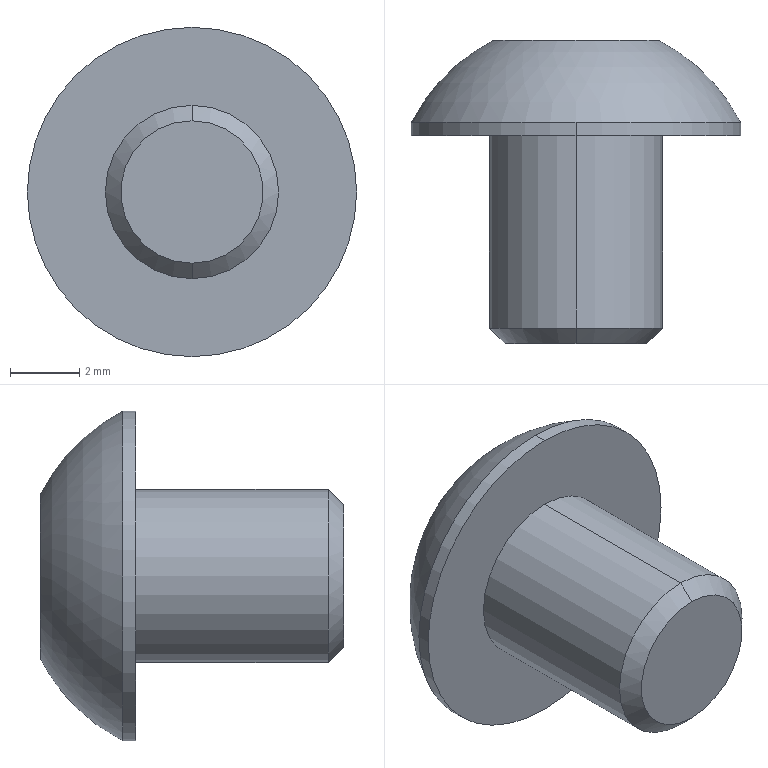Part | SolidWorks | features BaseBody 1 | 1 solid | 17 faces | box 9.5 x 8.75 x 9.5 mm | volume 242.513 mm3 | plane 10 | cylinder 4 | cone 2 | sphere 1 | commonest cylinder face diameters 5 x2 9.5 x2
STEP:
#1=CARTESIAN_POINT('',(0.,-6.,-2.055));
#2=VERTEX_POINT('',#1);
#3=CARTESIAN_POINT('',(0.,-6.,2.055));
#4=VERTEX_POINT('',#3);
#5=CARTESIAN_POINT('',(0.,-6.,0.));
#6=DIRECTION('',(0.,-1.,0.));
#7=DIRECTION('',(0.,0.,-1.));
#8=AXIS2_PLACEMENT_3D('',#5,#6,#7);
#9=CIRCLE('',#8,2.055);
#10=EDGE_CURVE('',#2,#4,#9,.T.);
#11=ORIENTED_EDGE('',*,*,#10,.F.);
#12=CARTESIAN_POINT('',(0.,-5.555,-2.5));
#13=VERTEX_POINT('',#12);
#14=CARTESIAN_POINT('',(0.,-6.,-2.055));
#15=DIRECTION('',(0.,0.7071,-0.7071));
#16=VECTOR('',#15,1000.);
#17=LINE('',#14,#16);
#18=EDGE_CURVE('',#2,#13,#17,.T.);
#19=ORIENTED_EDGE('',*,*,#18,.T.);
#20=CARTESIAN_POINT('',(0.,-5.555,2.5));
#21=VERTEX_POINT('',#20);
#22=CARTESIAN_POINT('',(0.,-5.555,0.));
#23=DIRECTION('',(0.,1.,0.));
#24=DIRECTION('',(0.,0.,-1.));
#25=AXIS2_PLACEMENT_3D('',#22,#23,#24);
#26=CIRCLE('',#25,2.5);
#27=EDGE_CURVE('',#21,#13,#26,.T.);
#28=ORIENTED_EDGE('',*,*,#27,.F.);
#29=CARTESIAN_POINT('',(0.,-6.,2.055));
#30=DIRECTION('',(0.,0.7071,0.7071));
#31=VECTOR('',#30,1000.);
#32=LINE('',#29,#31);
#33=EDGE_CURVE('',#4,#21,#32,.T.);
#34=ORIENTED_EDGE('',*,*,#33,.F.);
#35=EDGE_LOOP('',(#11,#19,#28,#34));
#36=FACE_OUTER_BOUND('',#35,.T.);
#37=CARTESIAN_POINT('',(0.,-6.,0.));
#38=DIRECTION('',(0.,1.,0.));
#39=DIRECTION('',(0.,0.,1.));
#40=AXIS2_PLACEMENT_3D('',#37,#38,#39);
#41=CONICAL_SURFACE('',#40,2.055,0.7854);
#42=ADVANCED_FACE('',(#36),#41,.T.);
#43=ORIENTED_EDGE('',*,*,#27,.T.);
#44=CARTESIAN_POINT('',(0.,0.,-2.5));
#45=VERTEX_POINT('',#44);
#46=CARTESIAN_POINT('',(0.,-6.,-2.5));
#47=DIRECTION('',(0.,1.,0.));
#48=VECTOR('',#47,1000.);
#49=LINE('',#46,#48);
#50=EDGE_CURVE('',#13,#45,#49,.T.);
#51=ORIENTED_EDGE('',*,*,#50,.T.);
#52=CARTESIAN_POINT('',(0.,0.,2.5));
#53=VERTEX_POINT('',#52);
#54=CARTESIAN_POINT('',(0.,0.,0.));
#55=DIRECTION('',(0.,-1.,0.));
#56=DIRECTION('',(0.,0.,1.));
#57=AXIS2_PLACEMENT_3D('',#54,#55,#56);
#58=CIRCLE('',#57,2.5);
#59=EDGE_CURVE('',#45,#53,#58,.T.);
#60=ORIENTED_EDGE('',*,*,#59,.T.);
#61=CARTESIAN_POINT('',(0.,-6.,2.5));
#62=DIRECTION('',(0.,1.,0.));
#63=VECTOR('',#62,1000.);
#64=LINE('',#61,#63);
#65=EDGE_CURVE('',#21,#53,#64,.T.);
#66=ORIENTED_EDGE('',*,*,#65,.F.);
#67=EDGE_LOOP('',(#43,#51,#60,#66));
#68=FACE_OUTER_BOUND('',#67,.T.);
#69=CARTESIAN_POINT('',(0.,-6.,0.));
#70=DIRECTION('',(0.,1.,0.));
#71=DIRECTION('',(0.,0.,1.));
#72=AXIS2_PLACEMENT_3D('',#69,#70,#71);
#73=CYLINDRICAL_SURFACE('',#72,2.5);
#74=ADVANCED_FACE('',(#68),#73,.T.);
#75=CARTESIAN_POINT('',(0.,0.38,-4.75));
#76=VERTEX_POINT('',#75);
#77=CARTESIAN_POINT('',(0.,0.38,4.75));
#78=VERTEX_POINT('',#77);
#79=CARTESIAN_POINT('',(0.,0.38,0.));
#80=DIRECTION('',(0.,-1.,0.));
#81=DIRECTION('',(0.,0.,-1.));
#82=AXIS2_PLACEMENT_3D('',#79,#80,#81);
#83=CIRCLE('',#82,4.75);
#84=EDGE_CURVE('',#76,#78,#83,.T.);
#85=ORIENTED_EDGE('',*,*,#84,.T.);
#86=CARTESIAN_POINT('',(0.,0.,4.75));
#87=VERTEX_POINT('',#86);
#88=CARTESIAN_POINT('',(0.,2.75,4.75));
#89=DIRECTION('',(0.,-1.,0.));
#90=VECTOR('',#89,1000.);
#91=LINE('',#88,#90);
#92=EDGE_CURVE('',#78,#87,#91,.T.);
#93=ORIENTED_EDGE('',*,*,#92,.T.);
#94=CARTESIAN_POINT('',(0.,0.,-4.75));
#95=VERTEX_POINT('',#94);
#96=CARTESIAN_POINT('',(0.,0.,0.));
#97=DIRECTION('',(0.,1.,0.));
#98=DIRECTION('',(0.,0.,1.));
#99=AXIS2_PLACEMENT_3D('',#96,#97,#98);
#100=CIRCLE('',#99,4.75);
#101=EDGE_CURVE('',#87,#95,#100,.T.);
#102=ORIENTED_EDGE('',*,*,#101,.T.);
#103=CARTESIAN_POINT('',(0.,2.75,-4.75));
#104=DIRECTION('',(0.,-1.,0.));
#105=VECTOR('',#104,1000.);
#106=LINE('',#103,#105);
#107=EDGE_CURVE('',#76,#95,#106,.T.);
#108=ORIENTED_EDGE('',*,*,#107,.F.);
#109=EDGE_LOOP('',(#85,#93,#102,#108));
#110=FACE_OUTER_BOUND('',#109,.T.);
#111=CARTESIAN_POINT('',(0.,2.75,0.));
#112=DIRECTION('',(0.,-1.,0.));
#113=DIRECTION('',(0.,0.,-1.));
#114=AXIS2_PLACEMENT_3D('',#111,#112,#113);
#115=CYLINDRICAL_SURFACE('',#114,4.75);
#116=ADVANCED_FACE('',(#110),#115,.T.);
#117=CARTESIAN_POINT('',(0.8862,2.75,1.535));
#118=VERTEX_POINT('',#117);
#119=CARTESIAN_POINT('',(1.772,2.75,0.));
#120=VERTEX_POINT('',#119);
#121=CARTESIAN_POINT('',(0.8862,2.75,1.535));
#122=DIRECTION('',(0.5,0.,-0.866));
#123=VECTOR('',#122,1000.);
#124=LINE('',#121,#123);
#125=EDGE_CURVE('',#118,#120,#124,.T.);
#126=ORIENTED_EDGE('',*,*,#125,.F.);
#127=CARTESIAN_POINT('',(-0.8862,2.75,1.535));
#128=VERTEX_POINT('',#127);
#129=CARTESIAN_POINT('',(-0.8862,2.75,1.535));
#130=DIRECTION('',(1.,0.,0.));
#131=VECTOR('',#130,1000.);
#132=LINE('',#129,#131);
#133=EDGE_CURVE('',#128,#118,#132,.T.);
#134=ORIENTED_EDGE('',*,*,#133,.F.);
#135=CARTESIAN_POINT('',(-1.772,2.75,0.));
#136=VERTEX_POINT('',#135);
#137=CARTESIAN_POINT('',(-1.772,2.75,0.));
#138=DIRECTION('',(0.5,0.,0.866));
#139=VECTOR('',#138,1000.);
#140=LINE('',#137,#139);
#141=EDGE_CURVE('',#136,#128,#140,.T.);
#142=ORIENTED_EDGE('',*,*,#141,.F.);
#143=CARTESIAN_POINT('',(-0.8862,2.75,-1.535));
#144=VERTEX_POINT('',#143);
#145=CARTESIAN_POINT('',(-0.8862,2.75,-1.535));
#146=DIRECTION('',(-0.5,0.,0.866));
#147=VECTOR('',#146,1000.);
#148=LINE('',#145,#147);
#149=EDGE_CURVE('',#144,#136,#148,.T.);
#150=ORIENTED_EDGE('',*,*,#149,.F.);
#151=CARTESIAN_POINT('',(0.8862,2.75,-1.535));
#152=VERTEX_POINT('',#151);
#153=CARTESIAN_POINT('',(0.8862,2.75,-1.535));
#154=DIRECTION('',(-1.,0.,0.));
#155=VECTOR('',#154,1000.);
#156=LINE('',#153,#155);
#157=EDGE_CURVE('',#152,#144,#156,.T.);
#158=ORIENTED_EDGE('',*,*,#157,.F.);
#159=CARTESIAN_POINT('',(1.772,2.75,0.));
#160=DIRECTION('',(-0.5,0.,-0.866));
#161=VECTOR('',#160,1000.);
#162=LINE('',#159,#161);
#163=EDGE_CURVE('',#120,#152,#162,.T.);
#164=ORIENTED_EDGE('',*,*,#163,.F.);
#165=EDGE_LOOP('',(#126,#134,#142,#150,#158,#164));
#166=FACE_BOUND('',#165,.T.);
#167=CARTESIAN_POINT('',(0.,2.75,-2.375));
#168=VERTEX_POINT('',#167);
#169=CARTESIAN_POINT('',(0.,2.75,2.375));
#170=VERTEX_POINT('',#169);
#171=CARTESIAN_POINT('',(0.,2.75,0.));
#172=DIRECTION('',(0.,-1.,0.));
#173=DIRECTION('',(0.,0.,-1.));
#174=AXIS2_PLACEMENT_3D('',#171,#172,#173);
#175=CIRCLE('',#174,2.375);
#176=EDGE_CURVE('',#168,#170,#175,.T.);
#177=ORIENTED_EDGE('',*,*,#176,.F.);
#178=CARTESIAN_POINT('',(0.,2.75,0.));
#179=DIRECTION('',(0.,-1.,0.));
#180=DIRECTION('',(0.,0.,-1.));
#181=AXIS2_PLACEMENT_3D('',#178,#179,#180);
#182=CIRCLE('',#181,2.375);
#183=EDGE_CURVE('',#170,#168,#182,.T.);
#184=ORIENTED_EDGE('',*,*,#183,.F.);
#185=EDGE_LOOP('',(#177,#184));
#186=FACE_OUTER_BOUND('',#185,.T.);
#187=CARTESIAN_POINT('',(0.,2.75,0.));
#188=DIRECTION('',(0.,1.,0.));
#189=DIRECTION('',(1.,0.,0.));
#190=AXIS2_PLACEMENT_3D('',#187,#188,#189);
#191=PLANE('',#190);
#192=ADVANCED_FACE('',(#166,#186),#191,.T.);
#193=ORIENTED_EDGE('',*,*,#125,.T.);
#194=CARTESIAN_POINT('',(1.772,1.19,0.));
#195=VERTEX_POINT('',#194);
#196=CARTESIAN_POINT('',(1.772,1.19,0.));
#197=DIRECTION('',(0.,1.,0.));
#198=VECTOR('',#197,1000.);
#199=LINE('',#196,#198);
#200=EDGE_CURVE('',#195,#120,#199,.T.);
#201=ORIENTED_EDGE('',*,*,#200,.F.);
#202=CARTESIAN_POINT('',(0.8862,1.19,1.535));
#203=VERTEX_POINT('',#202);
#204=CARTESIAN_POINT('',(0.8862,1.19,1.535));
#205=DIRECTION('',(0.5,0.,-0.866));
#206=VECTOR('',#205,1000.);
#207=LINE('',#204,#206);
#208=EDGE_CURVE('',#203,#195,#207,.T.);
#209=ORIENTED_EDGE('',*,*,#208,.F.);
#210=CARTESIAN_POINT('',(0.8862,1.19,1.535));
#211=DIRECTION('',(0.,1.,0.));
#212=VECTOR('',#211,1000.);
#213=LINE('',#210,#212);
#214=EDGE_CURVE('',#203,#118,#213,.T.);
#215=ORIENTED_EDGE('',*,*,#214,.T.);
#216=EDGE_LOOP('',(#193,#201,#209,#215));
#217=FACE_OUTER_BOUND('',#216,.T.);
#218=CARTESIAN_POINT('',(0.8862,1.19,1.535));
#219=DIRECTION('',(0.866,0.,0.5));
#220=DIRECTION('',(0.,-1.,0.));
#221=AXIS2_PLACEMENT_3D('',#218,#219,#220);
#222=PLANE('',#221);
#223=ADVANCED_FACE('',(#217),#222,.F.);
#224=ORIENTED_EDGE('',*,*,#133,.T.);
#225=ORIENTED_EDGE('',*,*,#214,.F.);
#226=CARTESIAN_POINT('',(-0.8862,1.19,1.535));
#227=VERTEX_POINT('',#226);
#228=CARTESIAN_POINT('',(-0.8862,1.19,1.535));
#229=DIRECTION('',(1.,0.,0.));
#230=VECTOR('',#229,1000.);
#231=LINE('',#228,#230);
#232=EDGE_CURVE('',#227,#203,#231,.T.);
#233=ORIENTED_EDGE('',*,*,#232,.F.);
#234=CARTESIAN_POINT('',(-0.8862,1.19,1.535));
#235=DIRECTION('',(0.,1.,0.));
#236=VECTOR('',#235,1000.);
#237=LINE('',#234,#236);
#238=EDGE_CURVE('',#227,#128,#237,.T.);
#239=ORIENTED_EDGE('',*,*,#238,.T.);
#240=EDGE_LOOP('',(#224,#225,#233,#239));
#241=FACE_OUTER_BOUND('',#240,.T.);
#242=CARTESIAN_POINT('',(-0.8862,1.19,1.535));
#243=DIRECTION('',(0.,0.,1.));
#244=DIRECTION('',(1.,0.,0.));
#245=AXIS2_PLACEMENT_3D('',#242,#243,#244);
#246=PLANE('',#245);
#247=ADVANCED_FACE('',(#241),#246,.F.);
#248=ORIENTED_EDGE('',*,*,#141,.T.);
#249=ORIENTED_EDGE('',*,*,#238,.F.);
#250=CARTESIAN_POINT('',(-1.772,1.19,0.));
#251=VERTEX_POINT('',#250);
#252=CARTESIAN_POINT('',(-1.772,1.19,0.));
#253=DIRECTION('',(0.5,0.,0.866));
#254=VECTOR('',#253,1000.);
#255=LINE('',#252,#254);
#256=EDGE_CURVE('',#251,#227,#255,.T.);
#257=ORIENTED_EDGE('',*,*,#256,.F.);
#258=CARTESIAN_POINT('',(-1.772,1.19,0.));
#259=DIRECTION('',(0.,1.,0.));
#260=VECTOR('',#259,1000.);
#261=LINE('',#258,#260);
#262=EDGE_CURVE('',#251,#136,#261,.T.);
#263=ORIENTED_EDGE('',*,*,#262,.T.);
#264=EDGE_LOOP('',(#248,#249,#257,#263));
#265=FACE_OUTER_BOUND('',#264,.T.);
#266=CARTESIAN_POINT('',(-1.772,1.19,0.));
#267=DIRECTION('',(-0.866,0.,0.5));
#268=DIRECTION('',(0.,1.,0.));
#269=AXIS2_PLACEMENT_3D('',#266,#267,#268);
#270=PLANE('',#269);
#271=ADVANCED_FACE('',(#265),#270,.F.);
#272=ORIENTED_EDGE('',*,*,#149,.T.);
#273=ORIENTED_EDGE('',*,*,#262,.F.);
#274=CARTESIAN_POINT('',(-0.8862,1.19,-1.535));
#275=VERTEX_POINT('',#274);
#276=CARTESIAN_POINT('',(-0.8862,1.19,-1.535));
#277=DIRECTION('',(-0.5,0.,0.866));
#278=VECTOR('',#277,1000.);
#279=LINE('',#276,#278);
#280=EDGE_CURVE('',#275,#251,#279,.T.);
#281=ORIENTED_EDGE('',*,*,#280,.F.);
#282=CARTESIAN_POINT('',(-0.8862,1.19,-1.535));
#283=DIRECTION('',(0.,1.,0.));
#284=VECTOR('',#283,1000.);
#285=LINE('',#282,#284);
#286=EDGE_CURVE('',#275,#144,#285,.T.);
#287=ORIENTED_EDGE('',*,*,#286,.T.);
#288=EDGE_LOOP('',(#272,#273,#281,#287));
#289=FACE_OUTER_BOUND('',#288,.T.);
#290=CARTESIAN_POINT('',(-0.8862,1.19,-1.535));
#291=DIRECTION('',(-0.866,0.,-0.5));
#292=DIRECTION('',(-0.5,0.,0.866));
#293=AXIS2_PLACEMENT_3D('',#290,#291,#292);
#294=PLANE('',#293);
#295=ADVANCED_FACE('',(#289),#294,.F.);
#296=ORIENTED_EDGE('',*,*,#157,.T.);
#297=ORIENTED_EDGE('',*,*,#286,.F.);
#298=CARTESIAN_POINT('',(0.8862,1.19,-1.535));
#299=VERTEX_POINT('',#298);
#300=CARTESIAN_POINT('',(0.8862,1.19,-1.535));
#301=DIRECTION('',(-1.,0.,0.));
#302=VECTOR('',#301,1000.);
#303=LINE('',#300,#302);
#304=EDGE_CURVE('',#299,#275,#303,.T.);
#305=ORIENTED_EDGE('',*,*,#304,.F.);
#306=CARTESIAN_POINT('',(0.8862,1.19,-1.535));
#307=DIRECTION('',(0.,1.,0.));
#308=VECTOR('',#307,1000.);
#309=LINE('',#306,#308);
#310=EDGE_CURVE('',#299,#152,#309,.T.);
#311=ORIENTED_EDGE('',*,*,#310,.T.);
#312=EDGE_LOOP('',(#296,#297,#305,#311));
#313=FACE_OUTER_BOUND('',#312,.T.);
#314=CARTESIAN_POINT('',(0.8862,1.19,-1.535));
#315=DIRECTION('',(0.,0.,-1.));
#316=DIRECTION('',(-1.,0.,0.));
#317=AXIS2_PLACEMENT_3D('',#314,#315,#316);
#318=PLANE('',#317);
#319=ADVANCED_FACE('',(#313),#318,.F.);
#320=ORIENTED_EDGE('',*,*,#163,.T.);
#321=ORIENTED_EDGE('',*,*,#310,.F.);
#322=CARTESIAN_POINT('',(1.772,1.19,0.));
#323=DIRECTION('',(-0.5,0.,-0.866));
#324=VECTOR('',#323,1000.);
#325=LINE('',#322,#324);
#326=EDGE_CURVE('',#195,#299,#325,.T.);
#327=ORIENTED_EDGE('',*,*,#326,.F.);
#328=ORIENTED_EDGE('',*,*,#200,.T.);
#329=EDGE_LOOP('',(#320,#321,#327,#328));
#330=FACE_OUTER_BOUND('',#329,.T.);
#331=CARTESIAN_POINT('',(1.772,1.19,0.));
#332=DIRECTION('',(0.866,0.,-0.5));
#333=DIRECTION('',(0.,-1.,0.));
#334=AXIS2_PLACEMENT_3D('',#331,#332,#333);
#335=PLANE('',#334);
#336=ADVANCED_FACE('',(#330),#335,.F.);
#337=ORIENTED_EDGE('',*,*,#208,.T.);
#338=ORIENTED_EDGE('',*,*,#326,.T.);
#339=ORIENTED_EDGE('',*,*,#304,.T.);
#340=ORIENTED_EDGE('',*,*,#280,.T.);
#341=ORIENTED_EDGE('',*,*,#256,.T.);
#342=ORIENTED_EDGE('',*,*,#232,.T.);
#343=EDGE_LOOP('',(#337,#338,#339,#340,#341,#342));
#344=FACE_OUTER_BOUND('',#343,.T.);
#345=CARTESIAN_POINT('',(0.,1.19,0.));
#346=DIRECTION('',(0.,1.,0.));
#347=DIRECTION('',(1.,0.,0.));
#348=AXIS2_PLACEMENT_3D('',#345,#346,#347);
#349=PLANE('',#348);
#350=ADVANCED_FACE('',(#344),#349,.T.);
#351=CARTESIAN_POINT('',(0.,-6.,0.));
#352=DIRECTION('',(0.,-1.,0.));
#353=DIRECTION('',(0.,0.,-1.));
#354=AXIS2_PLACEMENT_3D('',#351,#352,#353);
#355=CIRCLE('',#354,2.055);
#356=EDGE_CURVE('',#4,#2,#355,.T.);
#357=ORIENTED_EDGE('',*,*,#356,.T.);
#358=ORIENTED_EDGE('',*,*,#10,.T.);
#359=EDGE_LOOP('',(#357,#358));
#360=FACE_OUTER_BOUND('',#359,.T.);
#361=CARTESIAN_POINT('',(0.,-6.,0.));
#362=DIRECTION('',(0.,-1.,0.));
#363=DIRECTION('',(0.,0.,-1.));
#364=AXIS2_PLACEMENT_3D('',#361,#362,#363);
#365=PLANE('',#364);
#366=ADVANCED_FACE('',(#360),#365,.T.);
#367=CARTESIAN_POINT('',(0.,0.,0.));
#368=DIRECTION('',(0.,-1.,0.));
#369=DIRECTION('',(0.,0.,1.));
#370=AXIS2_PLACEMENT_3D('',#367,#368,#369);
#371=CIRCLE('',#370,2.5);
#372=EDGE_CURVE('',#53,#45,#371,.T.);
#373=ORIENTED_EDGE('',*,*,#372,.F.);
#374=ORIENTED_EDGE('',*,*,#59,.F.);
#375=EDGE_LOOP('',(#373,#374));
#376=FACE_BOUND('',#375,.T.);
#377=CARTESIAN_POINT('',(0.,0.,0.));
#378=DIRECTION('',(0.,1.,0.));
#379=DIRECTION('',(0.,0.,1.));
#380=AXIS2_PLACEMENT_3D('',#377,#378,#379);
#381=CIRCLE('',#380,4.75);
#382=EDGE_CURVE('',#95,#87,#381,.T.);
#383=ORIENTED_EDGE('',*,*,#382,.F.);
#384=ORIENTED_EDGE('',*,*,#101,.F.);
#385=EDGE_LOOP('',(#383,#384));
#386=FACE_OUTER_BOUND('',#385,.T.);
#387=CARTESIAN_POINT('',(0.,0.,0.));
#388=DIRECTION('',(0.,1.,0.));
#389=DIRECTION('',(1.,0.,0.));
#390=AXIS2_PLACEMENT_3D('',#387,#388,#389);
#391=PLANE('',#390);
#392=ADVANCED_FACE('',(#376,#386),#391,.F.);
#393=ORIENTED_EDGE('',*,*,#92,.F.);
#394=CARTESIAN_POINT('',(0.,0.38,0.));
#395=DIRECTION('',(0.,-1.,0.));
#396=DIRECTION('',(0.,0.,-1.));
#397=AXIS2_PLACEMENT_3D('',#394,#395,#396);
#398=CIRCLE('',#397,4.75);
#399=EDGE_CURVE('',#78,#76,#398,.T.);
#400=ORIENTED_EDGE('',*,*,#399,.T.);
#401=ORIENTED_EDGE('',*,*,#107,.T.);
#402=ORIENTED_EDGE('',*,*,#382,.T.);
#403=EDGE_LOOP('',(#393,#400,#401,#402));
#404=FACE_OUTER_BOUND('',#403,.T.);
#405=CARTESIAN_POINT('',(0.,2.75,0.));
#406=DIRECTION('',(0.,-1.,0.));
#407=DIRECTION('',(0.,0.,-1.));
#408=AXIS2_PLACEMENT_3D('',#405,#406,#407);
#409=CYLINDRICAL_SURFACE('',#408,4.75);
#410=ADVANCED_FACE('',(#404),#409,.T.);
#411=ORIENTED_EDGE('',*,*,#50,.F.);
#412=CARTESIAN_POINT('',(0.,-5.555,0.));
#413=DIRECTION('',(0.,1.,0.));
#414=DIRECTION('',(0.,0.,-1.));
#415=AXIS2_PLACEMENT_3D('',#412,#413,#414);
#416=CIRCLE('',#415,2.5);
#417=EDGE_CURVE('',#13,#21,#416,.T.);
#418=ORIENTED_EDGE('',*,*,#417,.T.);
#419=ORIENTED_EDGE('',*,*,#65,.T.);
#420=ORIENTED_EDGE('',*,*,#372,.T.);
#421=EDGE_LOOP('',(#411,#418,#419,#420));
#422=FACE_OUTER_BOUND('',#421,.T.);
#423=CARTESIAN_POINT('',(0.,-6.,0.));
#424=DIRECTION('',(0.,1.,0.));
#425=DIRECTION('',(0.,0.,1.));
#426=AXIS2_PLACEMENT_3D('',#423,#424,#425);
#427=CYLINDRICAL_SURFACE('',#426,2.5);
#428=ADVANCED_FACE('',(#422),#427,.T.);
#429=ORIENTED_EDGE('',*,*,#84,.F.);
#430=ORIENTED_EDGE('',*,*,#399,.F.);
#431=EDGE_LOOP('',(#429,#430));
#432=FACE_OUTER_BOUND('',#431,.T.);
#433=ORIENTED_EDGE('',*,*,#176,.T.);
#434=ORIENTED_EDGE('',*,*,#183,.T.);
#435=EDGE_LOOP('',(#433,#434));
#436=FACE_BOUND('',#435,.T.);
#437=CARTESIAN_POINT('',(0.,-2.005,0.));
#438=DIRECTION('',(0.,1.,0.));
#439=DIRECTION('',(1.,0.,0.));
#440=AXIS2_PLACEMENT_3D('',#437,#438,#439);
#441=SPHERICAL_SURFACE('',#440,5.315);
#442=ADVANCED_FACE('',(#432,#436),#441,.T.);
#443=ORIENTED_EDGE('',*,*,#18,.F.);
#444=ORIENTED_EDGE('',*,*,#356,.F.);
#445=ORIENTED_EDGE('',*,*,#33,.T.);
#446=ORIENTED_EDGE('',*,*,#417,.F.);
#447=EDGE_LOOP('',(#443,#444,#445,#446));
#448=FACE_OUTER_BOUND('',#447,.T.);
#449=CARTESIAN_POINT('',(0.,-6.,0.));
#450=DIRECTION('',(0.,1.,0.));
#451=DIRECTION('',(0.,0.,1.));
#452=AXIS2_PLACEMENT_3D('',#449,#450,#451);
#453=CONICAL_SURFACE('',#452,2.055,0.7854);
#454=ADVANCED_FACE('',(#448),#453,.T.);
#455=CLOSED_SHELL('',(#42,#74,#116,#192,#223,#247,#271,#295,#319,#336,#350,#366,#392,#410,#428,#442,#454));
#456=MANIFOLD_SOLID_BREP('',#455);
#457=CARTESIAN_POINT('',(0.,0.,0.));
#458=DIRECTION('',(0.,0.,1.));
#459=DIRECTION('',(1.,0.,0.));
#460=AXIS2_PLACEMENT_3D('',#457,#458,#459);
#461=(LENGTH_UNIT()NAMED_UNIT(*)SI_UNIT(.MILLI.,.METRE.));
#462=UNCERTAINTY_MEASURE_WITH_UNIT(LENGTH_MEASURE(0.00001),#461,'','');
#463=(NAMED_UNIT(*)PLANE_ANGLE_UNIT()SI_UNIT($,.RADIAN.));
#464=(NAMED_UNIT(*)SI_UNIT($,.STERADIAN.)SOLID_ANGLE_UNIT());
#465=(GEOMETRIC_REPRESENTATION_CONTEXT(3)GLOBAL_UNCERTAINTY_ASSIGNED_CONTEXT((#462))GLOBAL_UNIT_ASSIGNED_CONTEXT((#461,#463,#464))REPRESENTATION_CONTEXT('',''));
#466=ADVANCED_BREP_SHAPE_REPRESENTATION('',(#456,#460),#465);